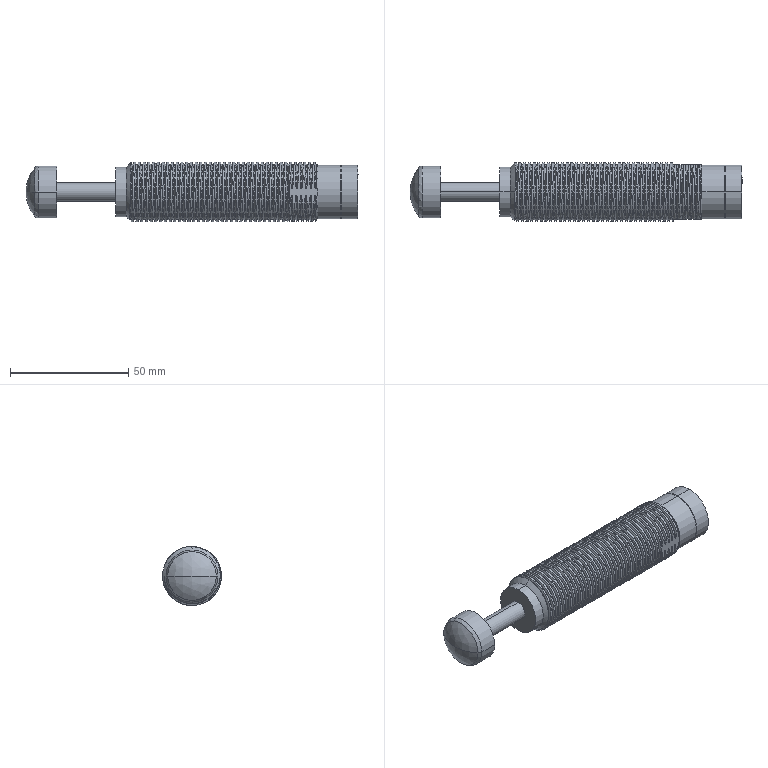Part | SolidWorks | features BaseBody 1 | 1 solid | 345 faces | box 140.5 x 24.8 x 25 mm | volume 51443 mm3 | plane 134 | cylinder 131 | spline 76 | cone 4 | commonest cylinder face diameters 25 x119 22 x4 22.8 x4 8 x2 21 x2